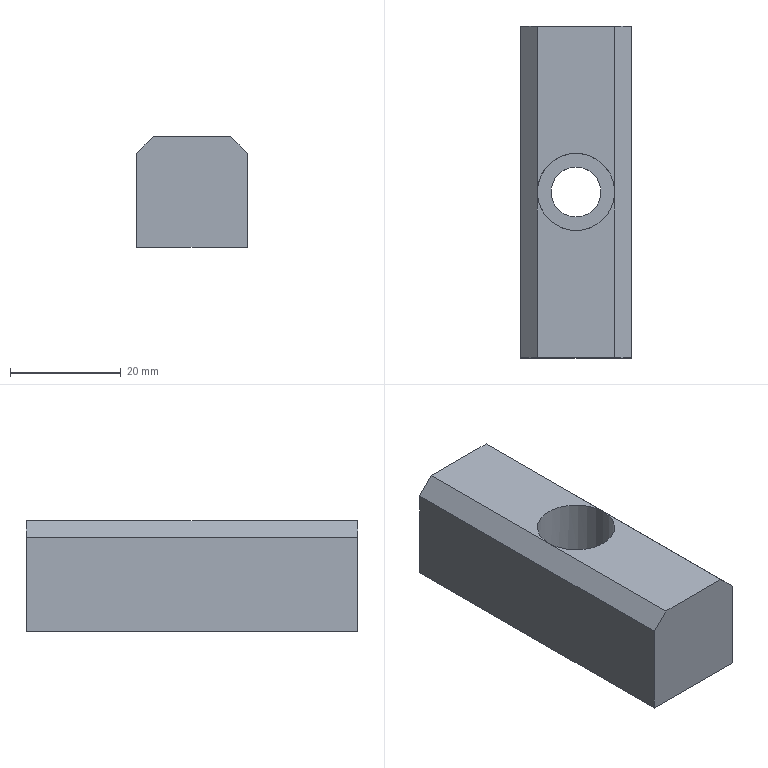Part | NX | features solid 2 | 1 solid | 12 faces | box 20 x 60 x 20 mm | volume 21284 mm3 | plane 10 | cylinder 2 | commonest cylinder face diameters 9 x1 14 x1
STEP:
#1=CARTESIAN_POINT('',(-177.,-45.,-368.));
#2=VERTEX_POINT('',#1);
#3=CARTESIAN_POINT('',(-163.,-45.,-368.));
#4=VERTEX_POINT('',#3);
#5=CARTESIAN_POINT('',(-170.,-45.,-368.));
#6=DIRECTION('',(1.,0.,0.));
#7=VECTOR('',#6,1000.);
#8=LINE('',#5,#7);
#9=EDGE_CURVE('',#2,#4,#8,.T.);
#10=ORIENTED_EDGE('',*,*,#9,.F.);
#11=CARTESIAN_POINT('',(-177.,-75.,-368.));
#12=VERTEX_POINT('',#11);
#13=CARTESIAN_POINT('',(-177.,-105.,-368.));
#14=DIRECTION('',(0.,-1.,0.));
#15=VECTOR('',#14,1000.);
#16=LINE('',#13,#15);
#17=EDGE_CURVE('',#2,#12,#16,.T.);
#18=ORIENTED_EDGE('',*,*,#17,.T.);
#19=CARTESIAN_POINT('',(-163.,-75.,-368.));
#20=VERTEX_POINT('',#19);
#21=CARTESIAN_POINT('',(-170.,-75.,-368.));
#22=DIRECTION('',(0.,0.,-1.));
#23=DIRECTION('',(0.,-1.,0.));
#24=AXIS2_PLACEMENT_3D('',#21,#22,#23);
#25=CIRCLE('',#24,7.);
#26=EDGE_CURVE('',#12,#20,#25,.T.);
#27=ORIENTED_EDGE('',*,*,#26,.T.);
#28=CARTESIAN_POINT('',(-163.,-105.,-368.));
#29=DIRECTION('',(0.,1.,0.));
#30=VECTOR('',#29,1000.);
#31=LINE('',#28,#30);
#32=EDGE_CURVE('',#20,#4,#31,.T.);
#33=ORIENTED_EDGE('',*,*,#32,.T.);
#34=EDGE_LOOP('',(#10,#18,#27,#33));
#35=FACE_BOUND('',#34,.T.);
#36=CARTESIAN_POINT('',(-170.,-105.,-368.));
#37=DIRECTION('',(0.,0.,-1.));
#38=DIRECTION('',(0.,-1.,0.));
#39=AXIS2_PLACEMENT_3D('',#36,#37,#38);
#40=PLANE('',#39);
#41=ADVANCED_FACE('',(#35),#40,.F.);
#42=CARTESIAN_POINT('',(-170.,-79.5,-388.));
#43=VERTEX_POINT('',#42);
#44=CARTESIAN_POINT('',(-170.,-75.,-388.));
#45=DIRECTION('',(0.,0.,-1.));
#46=DIRECTION('',(0.,-1.,0.));
#47=AXIS2_PLACEMENT_3D('',#44,#45,#46);
#48=CIRCLE('',#47,4.5);
#49=EDGE_CURVE('',#43,#43,#48,.T.);
#50=ORIENTED_EDGE('',*,*,#49,.F.);
#51=EDGE_LOOP('',(#50));
#52=FACE_BOUND('',#51,.T.);
#53=CARTESIAN_POINT('',(-180.,-105.,-388.));
#54=VERTEX_POINT('',#53);
#55=CARTESIAN_POINT('',(-160.,-105.,-388.));
#56=VERTEX_POINT('',#55);
#57=CARTESIAN_POINT('',(-170.,-105.,-388.));
#58=DIRECTION('',(1.,0.,0.));
#59=VECTOR('',#58,1000.);
#60=LINE('',#57,#59);
#61=EDGE_CURVE('',#54,#56,#60,.T.);
#62=ORIENTED_EDGE('',*,*,#61,.F.);
#63=CARTESIAN_POINT('',(-180.,-45.,-388.));
#64=VERTEX_POINT('',#63);
#65=CARTESIAN_POINT('',(-180.,-105.,-388.));
#66=DIRECTION('',(0.,1.,0.));
#67=VECTOR('',#66,1000.);
#68=LINE('',#65,#67);
#69=EDGE_CURVE('',#54,#64,#68,.T.);
#70=ORIENTED_EDGE('',*,*,#69,.T.);
#71=CARTESIAN_POINT('',(-160.,-45.,-388.));
#72=VERTEX_POINT('',#71);
#73=CARTESIAN_POINT('',(-170.,-45.,-388.));
#74=DIRECTION('',(1.,0.,0.));
#75=VECTOR('',#74,1000.);
#76=LINE('',#73,#75);
#77=EDGE_CURVE('',#64,#72,#76,.T.);
#78=ORIENTED_EDGE('',*,*,#77,.T.);
#79=CARTESIAN_POINT('',(-160.,-105.,-388.));
#80=DIRECTION('',(0.,1.,0.));
#81=VECTOR('',#80,1000.);
#82=LINE('',#79,#81);
#83=EDGE_CURVE('',#56,#72,#82,.T.);
#84=ORIENTED_EDGE('',*,*,#83,.F.);
#85=EDGE_LOOP('',(#62,#70,#78,#84));
#86=FACE_BOUND('',#85,.T.);
#87=CARTESIAN_POINT('',(-170.,-105.,-388.));
#88=DIRECTION('',(0.,0.,-1.));
#89=DIRECTION('',(0.,-1.,0.));
#90=AXIS2_PLACEMENT_3D('',#87,#88,#89);
#91=PLANE('',#90);
#92=ADVANCED_FACE('',(#52,#86),#91,.T.);
#93=CARTESIAN_POINT('',(-180.,-45.,-371.));
#94=VERTEX_POINT('',#93);
#95=CARTESIAN_POINT('',(-180.,-45.,-388.));
#96=DIRECTION('',(0.,0.,1.));
#97=VECTOR('',#96,1000.);
#98=LINE('',#95,#97);
#99=EDGE_CURVE('',#64,#94,#98,.T.);
#100=ORIENTED_EDGE('',*,*,#99,.T.);
#101=CARTESIAN_POINT('',(-183.5,-45.,-374.5));
#102=DIRECTION('',(0.7071,0.,0.7071));
#103=VECTOR('',#102,1000.);
#104=LINE('',#101,#103);
#105=EDGE_CURVE('',#94,#2,#104,.T.);
#106=ORIENTED_EDGE('',*,*,#105,.T.);
#107=ORIENTED_EDGE('',*,*,#9,.T.);
#108=CARTESIAN_POINT('',(-160.,-45.,-371.));
#109=VERTEX_POINT('',#108);
#110=CARTESIAN_POINT('',(-156.5,-45.,-374.5));
#111=DIRECTION('',(0.7071,0.,-0.7071));
#112=VECTOR('',#111,1000.);
#113=LINE('',#110,#112);
#114=EDGE_CURVE('',#4,#109,#113,.T.);
#115=ORIENTED_EDGE('',*,*,#114,.T.);
#116=CARTESIAN_POINT('',(-160.,-45.,-388.));
#117=DIRECTION('',(0.,0.,1.));
#118=VECTOR('',#117,1000.);
#119=LINE('',#116,#118);
#120=EDGE_CURVE('',#72,#109,#119,.T.);
#121=ORIENTED_EDGE('',*,*,#120,.F.);
#122=ORIENTED_EDGE('',*,*,#77,.F.);
#123=EDGE_LOOP('',(#100,#106,#107,#115,#121,#122));
#124=FACE_BOUND('',#123,.T.);
#125=CARTESIAN_POINT('',(-170.,-45.,-388.));
#126=DIRECTION('',(0.,1.,0.));
#127=DIRECTION('',(0.,0.,-1.));
#128=AXIS2_PLACEMENT_3D('',#125,#126,#127);
#129=PLANE('',#128);
#130=ADVANCED_FACE('',(#124),#129,.T.);
#131=CARTESIAN_POINT('',(-170.,-75.,-368.));
#132=DIRECTION('',(0.,0.,-1.));
#133=DIRECTION('',(0.,-1.,0.));
#134=AXIS2_PLACEMENT_3D('',#131,#132,#133);
#135=CIRCLE('',#134,7.);
#136=EDGE_CURVE('',#20,#12,#135,.T.);
#137=ORIENTED_EDGE('',*,*,#136,.T.);
#138=CARTESIAN_POINT('',(-177.,-105.,-368.));
#139=VERTEX_POINT('',#138);
#140=CARTESIAN_POINT('',(-177.,-105.,-368.));
#141=DIRECTION('',(0.,-1.,0.));
#142=VECTOR('',#141,1000.);
#143=LINE('',#140,#142);
#144=EDGE_CURVE('',#12,#139,#143,.T.);
#145=ORIENTED_EDGE('',*,*,#144,.T.);
#146=CARTESIAN_POINT('',(-163.,-105.,-368.));
#147=VERTEX_POINT('',#146);
#148=CARTESIAN_POINT('',(-170.,-105.,-368.));
#149=DIRECTION('',(1.,0.,0.));
#150=VECTOR('',#149,1000.);
#151=LINE('',#148,#150);
#152=EDGE_CURVE('',#139,#147,#151,.T.);
#153=ORIENTED_EDGE('',*,*,#152,.T.);
#154=CARTESIAN_POINT('',(-163.,-105.,-368.));
#155=DIRECTION('',(0.,1.,0.));
#156=VECTOR('',#155,1000.);
#157=LINE('',#154,#156);
#158=EDGE_CURVE('',#147,#20,#157,.T.);
#159=ORIENTED_EDGE('',*,*,#158,.T.);
#160=EDGE_LOOP('',(#137,#145,#153,#159));
#161=FACE_BOUND('',#160,.T.);
#162=CARTESIAN_POINT('',(-170.,-105.,-368.));
#163=DIRECTION('',(0.,0.,-1.));
#164=DIRECTION('',(0.,-1.,0.));
#165=AXIS2_PLACEMENT_3D('',#162,#163,#164);
#166=PLANE('',#165);
#167=ADVANCED_FACE('',(#161),#166,.F.);
#168=ORIENTED_EDGE('',*,*,#152,.F.);
#169=CARTESIAN_POINT('',(-180.,-105.,-371.));
#170=VERTEX_POINT('',#169);
#171=CARTESIAN_POINT('',(-183.5,-105.,-374.5));
#172=DIRECTION('',(-0.7071,0.,-0.7071));
#173=VECTOR('',#172,1000.);
#174=LINE('',#171,#173);
#175=EDGE_CURVE('',#139,#170,#174,.T.);
#176=ORIENTED_EDGE('',*,*,#175,.T.);
#177=CARTESIAN_POINT('',(-180.,-105.,-388.));
#178=DIRECTION('',(0.,0.,1.));
#179=VECTOR('',#178,1000.);
#180=LINE('',#177,#179);
#181=EDGE_CURVE('',#54,#170,#180,.T.);
#182=ORIENTED_EDGE('',*,*,#181,.F.);
#183=ORIENTED_EDGE('',*,*,#61,.T.);
#184=CARTESIAN_POINT('',(-160.,-105.,-371.));
#185=VERTEX_POINT('',#184);
#186=CARTESIAN_POINT('',(-160.,-105.,-388.));
#187=DIRECTION('',(0.,0.,1.));
#188=VECTOR('',#187,1000.);
#189=LINE('',#186,#188);
#190=EDGE_CURVE('',#56,#185,#189,.T.);
#191=ORIENTED_EDGE('',*,*,#190,.T.);
#192=CARTESIAN_POINT('',(-156.5,-105.,-374.5));
#193=DIRECTION('',(-0.7071,0.,0.7071));
#194=VECTOR('',#193,1000.);
#195=LINE('',#192,#194);
#196=EDGE_CURVE('',#185,#147,#195,.T.);
#197=ORIENTED_EDGE('',*,*,#196,.T.);
#198=EDGE_LOOP('',(#168,#176,#182,#183,#191,#197));
#199=FACE_BOUND('',#198,.T.);
#200=CARTESIAN_POINT('',(-170.,-105.,-388.));
#201=DIRECTION('',(0.,1.,0.));
#202=DIRECTION('',(0.,0.,-1.));
#203=AXIS2_PLACEMENT_3D('',#200,#201,#202);
#204=PLANE('',#203);
#205=ADVANCED_FACE('',(#199),#204,.F.);
#206=ORIENTED_EDGE('',*,*,#120,.T.);
#207=CARTESIAN_POINT('',(-160.,-105.,-371.));
#208=DIRECTION('',(0.,-1.,0.));
#209=VECTOR('',#208,1000.);
#210=LINE('',#207,#209);
#211=EDGE_CURVE('',#109,#185,#210,.T.);
#212=ORIENTED_EDGE('',*,*,#211,.T.);
#213=ORIENTED_EDGE('',*,*,#190,.F.);
#214=ORIENTED_EDGE('',*,*,#83,.T.);
#215=EDGE_LOOP('',(#206,#212,#213,#214));
#216=FACE_BOUND('',#215,.T.);
#217=CARTESIAN_POINT('',(-160.,-105.,-388.));
#218=DIRECTION('',(1.,0.,0.));
#219=DIRECTION('',(0.,-1.,0.));
#220=AXIS2_PLACEMENT_3D('',#217,#218,#219);
#221=PLANE('',#220);
#222=ADVANCED_FACE('',(#216),#221,.T.);
#223=ORIENTED_EDGE('',*,*,#181,.T.);
#224=CARTESIAN_POINT('',(-180.,-45.,-371.));
#225=DIRECTION('',(0.,1.,0.));
#226=VECTOR('',#225,1000.);
#227=LINE('',#224,#226);
#228=EDGE_CURVE('',#170,#94,#227,.T.);
#229=ORIENTED_EDGE('',*,*,#228,.T.);
#230=ORIENTED_EDGE('',*,*,#99,.F.);
#231=ORIENTED_EDGE('',*,*,#69,.F.);
#232=EDGE_LOOP('',(#223,#229,#230,#231));
#233=FACE_BOUND('',#232,.T.);
#234=CARTESIAN_POINT('',(-180.,-105.,-388.));
#235=DIRECTION('',(1.,0.,0.));
#236=DIRECTION('',(0.,-1.,0.));
#237=AXIS2_PLACEMENT_3D('',#234,#235,#236);
#238=PLANE('',#237);
#239=ADVANCED_FACE('',(#233),#238,.F.);
#240=ORIENTED_EDGE('',*,*,#49,.T.);
#241=EDGE_LOOP('',(#240));
#242=FACE_BOUND('',#241,.T.);
#243=CARTESIAN_POINT('',(-170.,-79.5,-378.));
#244=VERTEX_POINT('',#243);
#245=CARTESIAN_POINT('',(-170.,-75.,-378.));
#246=DIRECTION('',(0.,0.,-1.));
#247=DIRECTION('',(0.,-1.,0.));
#248=AXIS2_PLACEMENT_3D('',#245,#246,#247);
#249=CIRCLE('',#248,4.5);
#250=EDGE_CURVE('',#244,#244,#249,.T.);
#251=ORIENTED_EDGE('',*,*,#250,.F.);
#252=EDGE_LOOP('',(#251));
#253=FACE_BOUND('',#252,.T.);
#254=CARTESIAN_POINT('',(-170.,-75.,-418.));
#255=DIRECTION('',(0.,0.,-1.));
#256=DIRECTION('',(0.,1.,0.));
#257=AXIS2_PLACEMENT_3D('',#254,#255,#256);
#258=CYLINDRICAL_SURFACE('',#257,4.5);
#259=ADVANCED_FACE('',(#242,#253),#258,.F.);
#260=ORIENTED_EDGE('',*,*,#250,.T.);
#261=EDGE_LOOP('',(#260));
#262=FACE_BOUND('',#261,.T.);
#263=CARTESIAN_POINT('',(-170.,-82.,-378.));
#264=VERTEX_POINT('',#263);
#265=CARTESIAN_POINT('',(-170.,-75.,-378.));
#266=DIRECTION('',(0.,0.,-1.));
#267=DIRECTION('',(0.,-1.,0.));
#268=AXIS2_PLACEMENT_3D('',#265,#266,#267);
#269=CIRCLE('',#268,7.);
#270=EDGE_CURVE('',#264,#264,#269,.T.);
#271=ORIENTED_EDGE('',*,*,#270,.F.);
#272=EDGE_LOOP('',(#271));
#273=FACE_BOUND('',#272,.T.);
#274=CARTESIAN_POINT('',(-170.,-75.,-378.));
#275=DIRECTION('',(0.,0.,-1.));
#276=DIRECTION('',(0.,1.,0.));
#277=AXIS2_PLACEMENT_3D('',#274,#275,#276);
#278=PLANE('',#277);
#279=ADVANCED_FACE('',(#262,#273),#278,.F.);
#280=ORIENTED_EDGE('',*,*,#270,.T.);
#281=EDGE_LOOP('',(#280));
#282=FACE_BOUND('',#281,.T.);
#283=ORIENTED_EDGE('',*,*,#136,.F.);
#284=ORIENTED_EDGE('',*,*,#26,.F.);
#285=EDGE_LOOP('',(#283,#284));
#286=FACE_BOUND('',#285,.T.);
#287=CARTESIAN_POINT('',(-170.,-75.,-368.));
#288=DIRECTION('',(0.,0.,-1.));
#289=DIRECTION('',(0.,1.,0.));
#290=AXIS2_PLACEMENT_3D('',#287,#288,#289);
#291=CYLINDRICAL_SURFACE('',#290,7.);
#292=ADVANCED_FACE('',(#282,#286),#291,.F.);
#293=ORIENTED_EDGE('',*,*,#196,.F.);
#294=ORIENTED_EDGE('',*,*,#211,.F.);
#295=ORIENTED_EDGE('',*,*,#114,.F.);
#296=ORIENTED_EDGE('',*,*,#32,.F.);
#297=ORIENTED_EDGE('',*,*,#158,.F.);
#298=EDGE_LOOP('',(#293,#294,#295,#296,#297));
#299=FACE_BOUND('',#298,.T.);
#300=CARTESIAN_POINT('',(-163.,-105.,-368.));
#301=DIRECTION('',(0.7071,0.,0.7071));
#302=DIRECTION('',(-0.7071,0.,0.7071));
#303=AXIS2_PLACEMENT_3D('',#300,#301,#302);
#304=PLANE('',#303);
#305=ADVANCED_FACE('',(#299),#304,.T.);
#306=ORIENTED_EDGE('',*,*,#144,.F.);
#307=ORIENTED_EDGE('',*,*,#17,.F.);
#308=ORIENTED_EDGE('',*,*,#105,.F.);
#309=ORIENTED_EDGE('',*,*,#228,.F.);
#310=ORIENTED_EDGE('',*,*,#175,.F.);
#311=EDGE_LOOP('',(#306,#307,#308,#309,#310));
#312=FACE_BOUND('',#311,.T.);
#313=CARTESIAN_POINT('',(-180.,-105.,-371.));
#314=DIRECTION('',(0.7071,0.,-0.7071));
#315=DIRECTION('',(0.7071,0.,0.7071));
#316=AXIS2_PLACEMENT_3D('',#313,#314,#315);
#317=PLANE('',#316);
#318=ADVANCED_FACE('',(#312),#317,.F.);
#319=CLOSED_SHELL('',(#41,#92,#130,#167,#205,#222,#239,#259,#279,#292,#305,#318));
#320=MANIFOLD_SOLID_BREP('',#319);
#321=(LENGTH_UNIT()NAMED_UNIT(*)SI_UNIT(.MILLI.,.METRE.));
#322=UNCERTAINTY_MEASURE_WITH_UNIT(LENGTH_MEASURE(0.00001),#321,'','');
#323=(NAMED_UNIT(*)PLANE_ANGLE_UNIT()SI_UNIT($,.RADIAN.));
#324=(NAMED_UNIT(*)SI_UNIT($,.STERADIAN.)SOLID_ANGLE_UNIT());
#325=(GEOMETRIC_REPRESENTATION_CONTEXT(3)GLOBAL_UNCERTAINTY_ASSIGNED_CONTEXT((#322))GLOBAL_UNIT_ASSIGNED_CONTEXT((#321,#323,#324))REPRESENTATION_CONTEXT('',''));
#326=ADVANCED_BREP_SHAPE_REPRESENTATION('',(#320),#325);